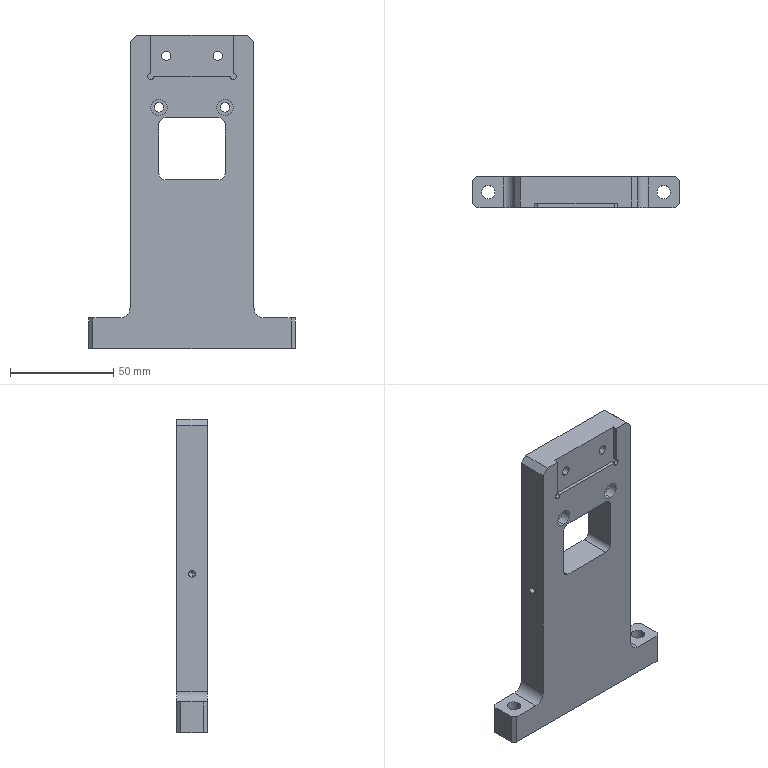Part | STEP file | PN_0042 | 1 solid | 70 faces | box 100 x 15 x 152 mm | volume 126808 mm3 | cylinder 36 | plane 28 | cone 6 | commonest cylinder face diameters 4.5 x8 8 x8 3 x4 5 x4 6 x4 6.5 x4